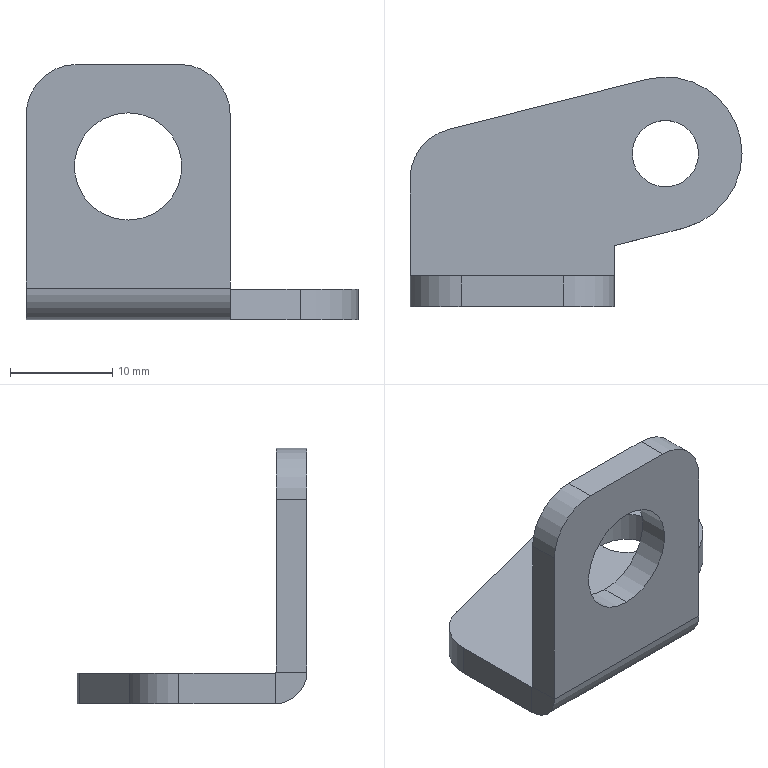Part | SolidWorks | features EdgeFlange 1, Fillet 1, FlatPattern 1, ICE 1, SMBaseFlange 1, SheetMetal 1 | 1 solid | 24 faces | box 32.5 x 22.5 x 25 mm | volume 2512 mm3 | plane 13 | cylinder 11 | commonest cylinder face diameters 10 x3 6.5 x2 10.5 x2 15 x2 0.2 x1 6.2 x1
STEP:
#1=CARTESIAN_POINT('',(0.,0.,6.75));
#2=VERTEX_POINT('',#1);
#3=CARTESIAN_POINT('',(0.,0.,17.25));
#4=VERTEX_POINT('',#3);
#5=CARTESIAN_POINT('',(0.,0.,12.));
#6=DIRECTION('',(0.,1.,0.));
#7=DIRECTION('',(0.,0.,1.));
#8=AXIS2_PLACEMENT_3D('',#5,#6,#7);
#9=CIRCLE('',#8,5.25);
#10=EDGE_CURVE('',#2,#4,#9,.T.);
#11=ORIENTED_EDGE('',*,*,#10,.F.);
#12=CARTESIAN_POINT('',(0.,3.,6.75));
#13=VERTEX_POINT('',#12);
#14=CARTESIAN_POINT('',(0.,-7.,6.75));
#15=DIRECTION('',(0.,1.,0.));
#16=VECTOR('',#15,1000.);
#17=LINE('',#14,#16);
#18=EDGE_CURVE('',#2,#13,#17,.T.);
#19=ORIENTED_EDGE('',*,*,#18,.T.);
#20=CARTESIAN_POINT('',(0.,3.,17.25));
#21=VERTEX_POINT('',#20);
#22=CARTESIAN_POINT('',(0.,3.,12.));
#23=DIRECTION('',(0.,1.,0.));
#24=DIRECTION('',(0.,0.,1.));
#25=AXIS2_PLACEMENT_3D('',#22,#23,#24);
#26=CIRCLE('',#25,5.25);
#27=EDGE_CURVE('',#13,#21,#26,.T.);
#28=ORIENTED_EDGE('',*,*,#27,.T.);
#29=CARTESIAN_POINT('',(0.,-7.,17.25));
#30=DIRECTION('',(0.,1.,0.));
#31=VECTOR('',#30,1000.);
#32=LINE('',#29,#31);
#33=EDGE_CURVE('',#4,#21,#32,.T.);
#34=ORIENTED_EDGE('',*,*,#33,.F.);
#35=EDGE_LOOP('',(#11,#19,#28,#34));
#36=FACE_OUTER_BOUND('',#35,.T.);
#37=CARTESIAN_POINT('',(0.,-7.,12.));
#38=DIRECTION('',(0.,1.,0.));
#39=DIRECTION('',(0.,0.,1.));
#40=AXIS2_PLACEMENT_3D('',#37,#38,#39);
#41=CYLINDRICAL_SURFACE('',#40,5.25);
#42=ADVANCED_FACE('',(#36),#41,.F.);
#43=CARTESIAN_POINT('',(11.75,15.,-3.));
#44=VERTEX_POINT('',#43);
#45=CARTESIAN_POINT('',(18.25,15.,-3.));
#46=VERTEX_POINT('',#45);
#47=CARTESIAN_POINT('',(15.,15.,-3.));
#48=DIRECTION('',(0.,0.,1.));
#49=DIRECTION('',(1.,0.,0.));
#50=AXIS2_PLACEMENT_3D('',#47,#48,#49);
#51=CIRCLE('',#50,3.25);
#52=EDGE_CURVE('',#44,#46,#51,.T.);
#53=ORIENTED_EDGE('',*,*,#52,.F.);
#54=CARTESIAN_POINT('',(11.75,15.,0.));
#55=VERTEX_POINT('',#54);
#56=CARTESIAN_POINT('',(11.75,15.,-3.));
#57=DIRECTION('',(0.,0.,1.));
#58=VECTOR('',#57,1000.);
#59=LINE('',#56,#58);
#60=EDGE_CURVE('',#44,#55,#59,.T.);
#61=ORIENTED_EDGE('',*,*,#60,.T.);
#62=CARTESIAN_POINT('',(18.25,15.,0.));
#63=VERTEX_POINT('',#62);
#64=CARTESIAN_POINT('',(15.,15.,0.));
#65=DIRECTION('',(0.,0.,1.));
#66=DIRECTION('',(1.,0.,0.));
#67=AXIS2_PLACEMENT_3D('',#64,#65,#66);
#68=CIRCLE('',#67,3.25);
#69=EDGE_CURVE('',#55,#63,#68,.T.);
#70=ORIENTED_EDGE('',*,*,#69,.T.);
#71=CARTESIAN_POINT('',(18.25,15.,-3.));
#72=DIRECTION('',(0.,0.,1.));
#73=VECTOR('',#72,1000.);
#74=LINE('',#71,#73);
#75=EDGE_CURVE('',#46,#63,#74,.T.);
#76=ORIENTED_EDGE('',*,*,#75,.F.);
#77=EDGE_LOOP('',(#53,#61,#70,#76));
#78=FACE_OUTER_BOUND('',#77,.T.);
#79=CARTESIAN_POINT('',(15.,15.,-3.));
#80=DIRECTION('',(0.,0.,1.));
#81=DIRECTION('',(1.,0.,0.));
#82=AXIS2_PLACEMENT_3D('',#79,#80,#81);
#83=CYLINDRICAL_SURFACE('',#82,3.25);
#84=ADVANCED_FACE('',(#78),#83,.F.);
#85=CARTESIAN_POINT('',(16.838,7.729,-3.));
#86=VERTEX_POINT('',#85);
#87=CARTESIAN_POINT('',(22.5,15.,-3.));
#88=VERTEX_POINT('',#87);
#89=CARTESIAN_POINT('',(15.,15.,-3.));
#90=DIRECTION('',(0.,0.,1.));
#91=DIRECTION('',(1.,0.,0.));
#92=AXIS2_PLACEMENT_3D('',#89,#90,#91);
#93=CIRCLE('',#92,7.5);
#94=EDGE_CURVE('',#86,#88,#93,.T.);
#95=ORIENTED_EDGE('',*,*,#94,.T.);
#96=CARTESIAN_POINT('',(22.5,15.,0.));
#97=VERTEX_POINT('',#96);
#98=CARTESIAN_POINT('',(22.5,15.,-3.));
#99=DIRECTION('',(0.,0.,1.));
#100=VECTOR('',#99,1000.);
#101=LINE('',#98,#100);
#102=EDGE_CURVE('',#88,#97,#101,.T.);
#103=ORIENTED_EDGE('',*,*,#102,.T.);
#104=CARTESIAN_POINT('',(16.838,7.729,0.));
#105=VERTEX_POINT('',#104);
#106=CARTESIAN_POINT('',(15.,15.,0.));
#107=DIRECTION('',(0.,0.,1.));
#108=DIRECTION('',(1.,0.,0.));
#109=AXIS2_PLACEMENT_3D('',#106,#107,#108);
#110=CIRCLE('',#109,7.5);
#111=EDGE_CURVE('',#105,#97,#110,.T.);
#112=ORIENTED_EDGE('',*,*,#111,.F.);
#113=CARTESIAN_POINT('',(16.838,7.729,-3.));
#114=DIRECTION('',(0.,0.,1.));
#115=VECTOR('',#114,1000.);
#116=LINE('',#113,#115);
#117=EDGE_CURVE('',#86,#105,#116,.T.);
#118=ORIENTED_EDGE('',*,*,#117,.F.);
#119=EDGE_LOOP('',(#95,#103,#112,#118));
#120=FACE_OUTER_BOUND('',#119,.T.);
#121=CARTESIAN_POINT('',(15.,15.,-3.));
#122=DIRECTION('',(0.,0.,1.));
#123=DIRECTION('',(1.,0.,0.));
#124=AXIS2_PLACEMENT_3D('',#121,#122,#123);
#125=CYLINDRICAL_SURFACE('',#124,7.5);
#126=ADVANCED_FACE('',(#120),#125,.T.);
#127=CARTESIAN_POINT('',(10.,3.1,0.));
#128=VERTEX_POINT('',#127);
#129=CARTESIAN_POINT('',(10.,6.,0.));
#130=VERTEX_POINT('',#129);
#131=CARTESIAN_POINT('',(10.,0.,0.));
#132=DIRECTION('',(0.,1.,0.));
#133=VECTOR('',#132,1000.);
#134=LINE('',#131,#133);
#135=EDGE_CURVE('',#128,#130,#134,.T.);
#136=ORIENTED_EDGE('',*,*,#135,.F.);
#137=CARTESIAN_POINT('',(10.,3.1,-3.));
#138=VERTEX_POINT('',#137);
#139=CARTESIAN_POINT('',(10.,3.1,0.));
#140=DIRECTION('',(0.,0.,-1.));
#141=VECTOR('',#140,1000.);
#142=LINE('',#139,#141);
#143=EDGE_CURVE('',#128,#138,#142,.T.);
#144=ORIENTED_EDGE('',*,*,#143,.T.);
#145=CARTESIAN_POINT('',(10.,6.,-3.));
#146=VERTEX_POINT('',#145);
#147=CARTESIAN_POINT('',(10.,0.,-3.));
#148=DIRECTION('',(0.,1.,0.));
#149=VECTOR('',#148,1000.);
#150=LINE('',#147,#149);
#151=EDGE_CURVE('',#138,#146,#150,.T.);
#152=ORIENTED_EDGE('',*,*,#151,.T.);
#153=CARTESIAN_POINT('',(10.,6.,-3.));
#154=DIRECTION('',(0.,0.,1.));
#155=VECTOR('',#154,1000.);
#156=LINE('',#153,#155);
#157=EDGE_CURVE('',#146,#130,#156,.T.);
#158=ORIENTED_EDGE('',*,*,#157,.T.);
#159=EDGE_LOOP('',(#136,#144,#152,#158));
#160=FACE_OUTER_BOUND('',#159,.T.);
#161=CARTESIAN_POINT('',(10.,0.,-3.));
#162=DIRECTION('',(1.,0.,0.));
#163=DIRECTION('',(0.,1.,0.));
#164=AXIS2_PLACEMENT_3D('',#161,#162,#163);
#165=PLANE('',#164);
#166=ADVANCED_FACE('',(#160),#165,.T.);
#167=CARTESIAN_POINT('',(15.,15.,-3.));
#168=DIRECTION('',(0.,0.,1.));
#169=DIRECTION('',(1.,0.,0.));
#170=AXIS2_PLACEMENT_3D('',#167,#168,#169);
#171=CIRCLE('',#170,3.25);
#172=EDGE_CURVE('',#46,#44,#171,.T.);
#173=ORIENTED_EDGE('',*,*,#172,.T.);
#174=ORIENTED_EDGE('',*,*,#52,.T.);
#175=EDGE_LOOP('',(#173,#174));
#176=FACE_BOUND('',#175,.T.);
#177=CARTESIAN_POINT('',(-10.,3.1,-3.));
#178=VERTEX_POINT('',#177);
#179=CARTESIAN_POINT('',(10.,3.1,-3.));
#180=DIRECTION('',(-1.,0.,0.));
#181=VECTOR('',#180,1000.);
#182=LINE('',#179,#181);
#183=EDGE_CURVE('',#138,#178,#182,.T.);
#184=ORIENTED_EDGE('',*,*,#183,.T.);
#185=CARTESIAN_POINT('',(-10.,12.522,-3.));
#186=VERTEX_POINT('',#185);
#187=CARTESIAN_POINT('',(-10.,0.,-3.));
#188=DIRECTION('',(0.,-1.,0.));
#189=VECTOR('',#188,1000.);
#190=LINE('',#187,#189);
#191=EDGE_CURVE('',#186,#178,#190,.T.);
#192=ORIENTED_EDGE('',*,*,#191,.F.);
#193=CARTESIAN_POINT('',(-6.225,17.37,-3.));
#194=VERTEX_POINT('',#193);
#195=CARTESIAN_POINT('',(-5.,12.522,-3.));
#196=DIRECTION('',(0.,0.,1.));
#197=DIRECTION('',(1.,0.,0.));
#198=AXIS2_PLACEMENT_3D('',#195,#196,#197);
#199=CIRCLE('',#198,5.);
#200=EDGE_CURVE('',#194,#186,#199,.T.);
#201=ORIENTED_EDGE('',*,*,#200,.F.);
#202=CARTESIAN_POINT('',(13.162,22.271,-3.));
#203=VERTEX_POINT('',#202);
#204=CARTESIAN_POINT('',(-6.225,17.37,-3.));
#205=DIRECTION('',(-0.9695,-0.2451,0.));
#206=VECTOR('',#205,1000.);
#207=LINE('',#204,#206);
#208=EDGE_CURVE('',#203,#194,#207,.T.);
#209=ORIENTED_EDGE('',*,*,#208,.F.);
#210=CARTESIAN_POINT('',(15.,15.,-3.));
#211=DIRECTION('',(0.,0.,1.));
#212=DIRECTION('',(1.,0.,0.));
#213=AXIS2_PLACEMENT_3D('',#210,#211,#212);
#214=CIRCLE('',#213,7.5);
#215=EDGE_CURVE('',#88,#203,#214,.T.);
#216=ORIENTED_EDGE('',*,*,#215,.F.);
#217=ORIENTED_EDGE('',*,*,#94,.F.);
#218=CARTESIAN_POINT('',(10.,6.,-3.));
#219=DIRECTION('',(0.9695,0.2451,0.));
#220=VECTOR('',#219,1000.);
#221=LINE('',#218,#220);
#222=EDGE_CURVE('',#146,#86,#221,.T.);
#223=ORIENTED_EDGE('',*,*,#222,.F.);
#224=ORIENTED_EDGE('',*,*,#151,.F.);
#225=EDGE_LOOP('',(#184,#192,#201,#209,#216,#217,#223,#224));
#226=FACE_OUTER_BOUND('',#225,.T.);
#227=CARTESIAN_POINT('',(-5.,12.522,-3.));
#228=DIRECTION('',(0.,0.,1.));
#229=DIRECTION('',(1.,0.,0.));
#230=AXIS2_PLACEMENT_3D('',#227,#228,#229);
#231=PLANE('',#230);
#232=ADVANCED_FACE('',(#176,#226),#231,.F.);
#233=CARTESIAN_POINT('',(15.,15.,0.));
#234=DIRECTION('',(0.,0.,1.));
#235=DIRECTION('',(1.,0.,0.));
#236=AXIS2_PLACEMENT_3D('',#233,#234,#235);
#237=CIRCLE('',#236,3.25);
#238=EDGE_CURVE('',#63,#55,#237,.T.);
#239=ORIENTED_EDGE('',*,*,#238,.F.);
#240=ORIENTED_EDGE('',*,*,#69,.F.);
#241=EDGE_LOOP('',(#239,#240));
#242=FACE_BOUND('',#241,.T.);
#243=CARTESIAN_POINT('',(-10.,12.522,0.));
#244=VERTEX_POINT('',#243);
#245=CARTESIAN_POINT('',(-10.,3.1,0.));
#246=VERTEX_POINT('',#245);
#247=CARTESIAN_POINT('',(-10.,0.,0.));
#248=DIRECTION('',(0.,-1.,0.));
#249=VECTOR('',#248,1000.);
#250=LINE('',#247,#249);
#251=EDGE_CURVE('',#244,#246,#250,.T.);
#252=ORIENTED_EDGE('',*,*,#251,.T.);
#253=CARTESIAN_POINT('',(10.,3.1,0.));
#254=DIRECTION('',(-1.,0.,0.));
#255=VECTOR('',#254,1000.);
#256=LINE('',#253,#255);
#257=EDGE_CURVE('',#128,#246,#256,.T.);
#258=ORIENTED_EDGE('',*,*,#257,.F.);
#259=ORIENTED_EDGE('',*,*,#135,.T.);
#260=CARTESIAN_POINT('',(10.,6.,0.));
#261=DIRECTION('',(0.9695,0.2451,0.));
#262=VECTOR('',#261,1000.);
#263=LINE('',#260,#262);
#264=EDGE_CURVE('',#130,#105,#263,.T.);
#265=ORIENTED_EDGE('',*,*,#264,.T.);
#266=ORIENTED_EDGE('',*,*,#111,.T.);
#267=CARTESIAN_POINT('',(13.162,22.271,0.));
#268=VERTEX_POINT('',#267);
#269=CARTESIAN_POINT('',(15.,15.,0.));
#270=DIRECTION('',(0.,0.,1.));
#271=DIRECTION('',(1.,0.,0.));
#272=AXIS2_PLACEMENT_3D('',#269,#270,#271);
#273=CIRCLE('',#272,7.5);
#274=EDGE_CURVE('',#97,#268,#273,.T.);
#275=ORIENTED_EDGE('',*,*,#274,.T.);
#276=CARTESIAN_POINT('',(-6.225,17.37,0.));
#277=VERTEX_POINT('',#276);
#278=CARTESIAN_POINT('',(-6.225,17.37,0.));
#279=DIRECTION('',(-0.9695,-0.2451,0.));
#280=VECTOR('',#279,1000.);
#281=LINE('',#278,#280);
#282=EDGE_CURVE('',#268,#277,#281,.T.);
#283=ORIENTED_EDGE('',*,*,#282,.T.);
#284=CARTESIAN_POINT('',(-5.,12.522,0.));
#285=DIRECTION('',(0.,0.,1.));
#286=DIRECTION('',(1.,0.,0.));
#287=AXIS2_PLACEMENT_3D('',#284,#285,#286);
#288=CIRCLE('',#287,5.);
#289=EDGE_CURVE('',#277,#244,#288,.T.);
#290=ORIENTED_EDGE('',*,*,#289,.T.);
#291=EDGE_LOOP('',(#252,#258,#259,#265,#266,#275,#283,#290));
#292=FACE_OUTER_BOUND('',#291,.T.);
#293=CARTESIAN_POINT('',(-5.,12.522,0.));
#294=DIRECTION('',(0.,0.,1.));
#295=DIRECTION('',(1.,0.,0.));
#296=AXIS2_PLACEMENT_3D('',#293,#294,#295);
#297=PLANE('',#296);
#298=ADVANCED_FACE('',(#242,#292),#297,.T.);
#299=CARTESIAN_POINT('',(-10.,3.1,0.));
#300=DIRECTION('',(0.,0.,-1.));
#301=VECTOR('',#300,1000.);
#302=LINE('',#299,#301);
#303=EDGE_CURVE('',#246,#178,#302,.T.);
#304=ORIENTED_EDGE('',*,*,#303,.F.);
#305=ORIENTED_EDGE('',*,*,#251,.F.);
#306=CARTESIAN_POINT('',(-10.,12.522,-3.));
#307=DIRECTION('',(0.,0.,1.));
#308=VECTOR('',#307,1000.);
#309=LINE('',#306,#308);
#310=EDGE_CURVE('',#186,#244,#309,.T.);
#311=ORIENTED_EDGE('',*,*,#310,.F.);
#312=ORIENTED_EDGE('',*,*,#191,.T.);
#313=EDGE_LOOP('',(#304,#305,#311,#312));
#314=FACE_OUTER_BOUND('',#313,.T.);
#315=CARTESIAN_POINT('',(-10.,0.,-3.));
#316=DIRECTION('',(-1.,0.,0.));
#317=DIRECTION('',(0.,0.,1.));
#318=AXIS2_PLACEMENT_3D('',#315,#316,#317);
#319=PLANE('',#318);
#320=ADVANCED_FACE('',(#314),#319,.T.);
#321=ORIENTED_EDGE('',*,*,#289,.F.);
#322=CARTESIAN_POINT('',(-6.225,17.37,-3.));
#323=DIRECTION('',(0.,0.,1.));
#324=VECTOR('',#323,1000.);
#325=LINE('',#322,#324);
#326=EDGE_CURVE('',#194,#277,#325,.T.);
#327=ORIENTED_EDGE('',*,*,#326,.F.);
#328=ORIENTED_EDGE('',*,*,#200,.T.);
#329=ORIENTED_EDGE('',*,*,#310,.T.);
#330=EDGE_LOOP('',(#321,#327,#328,#329));
#331=FACE_OUTER_BOUND('',#330,.T.);
#332=CARTESIAN_POINT('',(-5.,12.522,-3.));
#333=DIRECTION('',(0.,0.,1.));
#334=DIRECTION('',(1.,0.,0.));
#335=AXIS2_PLACEMENT_3D('',#332,#333,#334);
#336=CYLINDRICAL_SURFACE('',#335,5.);
#337=ADVANCED_FACE('',(#331),#336,.T.);
#338=ORIENTED_EDGE('',*,*,#282,.F.);
#339=CARTESIAN_POINT('',(13.162,22.271,-3.));
#340=DIRECTION('',(0.,0.,1.));
#341=VECTOR('',#340,1000.);
#342=LINE('',#339,#341);
#343=EDGE_CURVE('',#203,#268,#342,.T.);
#344=ORIENTED_EDGE('',*,*,#343,.F.);
#345=ORIENTED_EDGE('',*,*,#208,.T.);
#346=ORIENTED_EDGE('',*,*,#326,.T.);
#347=EDGE_LOOP('',(#338,#344,#345,#346));
#348=FACE_OUTER_BOUND('',#347,.T.);
#349=CARTESIAN_POINT('',(-6.225,17.37,-3.));
#350=DIRECTION('',(-0.2451,0.9695,0.));
#351=DIRECTION('',(-0.9695,-0.2451,0.));
#352=AXIS2_PLACEMENT_3D('',#349,#350,#351);
#353=PLANE('',#352);
#354=ADVANCED_FACE('',(#348),#353,.T.);
#355=ORIENTED_EDGE('',*,*,#102,.F.);
#356=ORIENTED_EDGE('',*,*,#215,.T.);
#357=ORIENTED_EDGE('',*,*,#343,.T.);
#358=ORIENTED_EDGE('',*,*,#274,.F.);
#359=EDGE_LOOP('',(#355,#356,#357,#358));
#360=FACE_OUTER_BOUND('',#359,.T.);
#361=CARTESIAN_POINT('',(15.,15.,-3.));
#362=DIRECTION('',(0.,0.,1.));
#363=DIRECTION('',(1.,0.,0.));
#364=AXIS2_PLACEMENT_3D('',#361,#362,#363);
#365=CYLINDRICAL_SURFACE('',#364,7.5);
#366=ADVANCED_FACE('',(#360),#365,.T.);
#367=ORIENTED_EDGE('',*,*,#264,.F.);
#368=ORIENTED_EDGE('',*,*,#157,.F.);
#369=ORIENTED_EDGE('',*,*,#222,.T.);
#370=ORIENTED_EDGE('',*,*,#117,.T.);
#371=EDGE_LOOP('',(#367,#368,#369,#370));
#372=FACE_OUTER_BOUND('',#371,.T.);
#373=CARTESIAN_POINT('',(10.,6.,-3.));
#374=DIRECTION('',(0.2451,-0.9695,0.));
#375=DIRECTION('',(0.9695,0.2451,0.));
#376=AXIS2_PLACEMENT_3D('',#373,#374,#375);
#377=PLANE('',#376);
#378=ADVANCED_FACE('',(#372),#377,.T.);
#379=ORIENTED_EDGE('',*,*,#60,.F.);
#380=ORIENTED_EDGE('',*,*,#172,.F.);
#381=ORIENTED_EDGE('',*,*,#75,.T.);
#382=ORIENTED_EDGE('',*,*,#238,.T.);
#383=EDGE_LOOP('',(#379,#380,#381,#382));
#384=FACE_OUTER_BOUND('',#383,.T.);
#385=CARTESIAN_POINT('',(15.,15.,-3.));
#386=DIRECTION('',(0.,0.,1.));
#387=DIRECTION('',(1.,0.,0.));
#388=AXIS2_PLACEMENT_3D('',#385,#386,#387);
#389=CYLINDRICAL_SURFACE('',#388,3.25);
#390=ADVANCED_FACE('',(#384),#389,.F.);
#391=CARTESIAN_POINT('',(-10.,3.,0.1));
#392=VERTEX_POINT('',#391);
#393=CARTESIAN_POINT('',(-10.,0.,0.1));
#394=VERTEX_POINT('',#393);
#395=CARTESIAN_POINT('',(-10.,0.,0.1));
#396=DIRECTION('',(0.,-1.,0.));
#397=VECTOR('',#396,1000.);
#398=LINE('',#395,#397);
#399=EDGE_CURVE('',#392,#394,#398,.T.);
#400=ORIENTED_EDGE('',*,*,#399,.F.);
#401=CARTESIAN_POINT('',(-10.,3.1,0.1));
#402=DIRECTION('',(-1.,0.,0.));
#403=DIRECTION('',(0.,0.,-1.));
#404=AXIS2_PLACEMENT_3D('',#401,#402,#403);
#405=CIRCLE('',#404,0.1);
#406=EDGE_CURVE('',#246,#392,#405,.T.);
#407=ORIENTED_EDGE('',*,*,#406,.F.);
#408=ORIENTED_EDGE('',*,*,#303,.T.);
#409=CARTESIAN_POINT('',(-10.,3.1,0.1));
#410=DIRECTION('',(-1.,0.,0.));
#411=DIRECTION('',(0.,0.,-1.));
#412=AXIS2_PLACEMENT_3D('',#409,#410,#411);
#413=CIRCLE('',#412,3.1);
#414=EDGE_CURVE('',#178,#394,#413,.T.);
#415=ORIENTED_EDGE('',*,*,#414,.T.);
#416=EDGE_LOOP('',(#400,#407,#408,#415));
#417=FACE_OUTER_BOUND('',#416,.T.);
#418=CARTESIAN_POINT('',(-10.,3.1,0.1));
#419=DIRECTION('',(-1.,0.,0.));
#420=DIRECTION('',(0.,0.,1.));
#421=AXIS2_PLACEMENT_3D('',#418,#419,#420);
#422=PLANE('',#421);
#423=ADVANCED_FACE('',(#417),#422,.T.);
#424=CARTESIAN_POINT('',(10.,3.,0.1));
#425=VERTEX_POINT('',#424);
#426=CARTESIAN_POINT('',(10.,3.1,0.1));
#427=DIRECTION('',(1.,0.,0.));
#428=DIRECTION('',(0.,0.,-1.));
#429=AXIS2_PLACEMENT_3D('',#426,#427,#428);
#430=CIRCLE('',#429,0.1);
#431=EDGE_CURVE('',#425,#128,#430,.T.);
#432=ORIENTED_EDGE('',*,*,#431,.F.);
#433=CARTESIAN_POINT('',(10.,0.,0.1));
#434=VERTEX_POINT('',#433);
#435=CARTESIAN_POINT('',(10.,3.,0.1));
#436=DIRECTION('',(0.,-1.,0.));
#437=VECTOR('',#436,1000.);
#438=LINE('',#435,#437);
#439=EDGE_CURVE('',#425,#434,#438,.T.);
#440=ORIENTED_EDGE('',*,*,#439,.T.);
#441=CARTESIAN_POINT('',(10.,3.1,0.1));
#442=DIRECTION('',(1.,0.,0.));
#443=DIRECTION('',(0.,0.,-1.));
#444=AXIS2_PLACEMENT_3D('',#441,#442,#443);
#445=CIRCLE('',#444,3.1);
#446=EDGE_CURVE('',#434,#138,#445,.T.);
#447=ORIENTED_EDGE('',*,*,#446,.T.);
#448=ORIENTED_EDGE('',*,*,#143,.F.);
#449=EDGE_LOOP('',(#432,#440,#447,#448));
#450=FACE_OUTER_BOUND('',#449,.T.);
#451=CARTESIAN_POINT('',(10.,3.1,0.1));
#452=DIRECTION('',(-1.,0.,0.));
#453=DIRECTION('',(0.,0.,1.));
#454=AXIS2_PLACEMENT_3D('',#451,#452,#453);
#455=PLANE('',#454);
#456=ADVANCED_FACE('',(#450),#455,.F.);
#457=ORIENTED_EDGE('',*,*,#183,.F.);
#458=ORIENTED_EDGE('',*,*,#446,.F.);
#459=CARTESIAN_POINT('',(-10.,0.,0.1));
#460=DIRECTION('',(-1.,0.,0.));
#461=VECTOR('',#460,1000.);
#462=LINE('',#459,#461);
#463=EDGE_CURVE('',#434,#394,#462,.T.);
#464=ORIENTED_EDGE('',*,*,#463,.T.);
#465=ORIENTED_EDGE('',*,*,#414,.F.);
#466=EDGE_LOOP('',(#457,#458,#464,#465));
#467=FACE_OUTER_BOUND('',#466,.T.);
#468=CARTESIAN_POINT('',(10.,3.1,0.1));
#469=DIRECTION('',(1.,0.,0.));
#470=DIRECTION('',(0.,-1.,0.));
#471=AXIS2_PLACEMENT_3D('',#468,#469,#470);
#472=CYLINDRICAL_SURFACE('',#471,3.1);
#473=ADVANCED_FACE('',(#467),#472,.T.);
#474=ORIENTED_EDGE('',*,*,#257,.T.);
#475=ORIENTED_EDGE('',*,*,#406,.T.);
#476=CARTESIAN_POINT('',(-10.,3.,0.1));
#477=DIRECTION('',(1.,0.,0.));
#478=VECTOR('',#477,1000.);
#479=LINE('',#476,#478);
#480=EDGE_CURVE('',#392,#425,#479,.T.);
#481=ORIENTED_EDGE('',*,*,#480,.T.);
#482=ORIENTED_EDGE('',*,*,#431,.T.);
#483=EDGE_LOOP('',(#474,#475,#481,#482));
#484=FACE_OUTER_BOUND('',#483,.T.);
#485=CARTESIAN_POINT('',(10.,3.1,0.1));
#486=DIRECTION('',(1.,0.,0.));
#487=DIRECTION('',(0.,-1.,0.));
#488=AXIS2_PLACEMENT_3D('',#485,#486,#487);
#489=CYLINDRICAL_SURFACE('',#488,0.1);
#490=ADVANCED_FACE('',(#484),#489,.F.);
#491=CARTESIAN_POINT('',(-10.,0.,17.));
#492=VERTEX_POINT('',#491);
#493=CARTESIAN_POINT('',(-10.,0.,0.));
#494=DIRECTION('',(0.,0.,-1.));
#495=VECTOR('',#494,1000.);
#496=LINE('',#493,#495);
#497=EDGE_CURVE('',#492,#394,#496,.T.);
#498=ORIENTED_EDGE('',*,*,#497,.F.);
#499=CARTESIAN_POINT('',(-10.,3.,17.));
#500=VERTEX_POINT('',#499);
#501=CARTESIAN_POINT('',(-10.,0.,17.));
#502=DIRECTION('',(0.,1.,0.));
#503=VECTOR('',#502,1000.);
#504=LINE('',#501,#503);
#505=EDGE_CURVE('',#492,#500,#504,.T.);
#506=ORIENTED_EDGE('',*,*,#505,.T.);
#507=CARTESIAN_POINT('',(-10.,3.,0.));
#508=DIRECTION('',(0.,0.,-1.));
#509=VECTOR('',#508,1000.);
#510=LINE('',#507,#509);
#511=EDGE_CURVE('',#500,#392,#510,.T.);
#512=ORIENTED_EDGE('',*,*,#511,.T.);
#513=ORIENTED_EDGE('',*,*,#399,.T.);
#514=EDGE_LOOP('',(#498,#506,#512,#513));
#515=FACE_OUTER_BOUND('',#514,.T.);
#516=CARTESIAN_POINT('',(-10.,0.,0.));
#517=DIRECTION('',(1.,0.,0.));
#518=DIRECTION('',(0.,0.,-1.));
#519=AXIS2_PLACEMENT_3D('',#516,#517,#518);
#520=PLANE('',#519);
#521=ADVANCED_FACE('',(#515),#520,.F.);
#522=CARTESIAN_POINT('',(10.,3.,17.));
#523=VERTEX_POINT('',#522);
#524=CARTESIAN_POINT('',(10.,3.,22.));
#525=DIRECTION('',(0.,0.,1.));
#526=VECTOR('',#525,1000.);
#527=LINE('',#524,#526);
#528=EDGE_CURVE('',#425,#523,#527,.T.);
#529=ORIENTED_EDGE('',*,*,#528,.T.);
#530=CARTESIAN_POINT('',(10.,0.,17.));
#531=VERTEX_POINT('',#530);
#532=CARTESIAN_POINT('',(10.,0.,17.));
#533=DIRECTION('',(0.,-1.,0.));
#534=VECTOR('',#533,1000.);
#535=LINE('',#532,#534);
#536=EDGE_CURVE('',#523,#531,#535,.T.);
#537=ORIENTED_EDGE('',*,*,#536,.T.);
#538=CARTESIAN_POINT('',(10.,0.,0.));
#539=DIRECTION('',(0.,0.,1.));
#540=VECTOR('',#539,1000.);
#541=LINE('',#538,#540);
#542=EDGE_CURVE('',#434,#531,#541,.T.);
#543=ORIENTED_EDGE('',*,*,#542,.F.);
#544=ORIENTED_EDGE('',*,*,#439,.F.);
#545=EDGE_LOOP('',(#529,#537,#543,#544));
#546=FACE_OUTER_BOUND('',#545,.T.);
#547=CARTESIAN_POINT('',(10.,0.,22.));
#548=DIRECTION('',(-1.,0.,0.));
#549=DIRECTION('',(0.,0.,1.));
#550=AXIS2_PLACEMENT_3D('',#547,#548,#549);
#551=PLANE('',#550);
#552=ADVANCED_FACE('',(#546),#551,.F.);
#553=CARTESIAN_POINT('',(0.,0.,12.));
#554=DIRECTION('',(0.,1.,0.));
#555=DIRECTION('',(0.,0.,1.));
#556=AXIS2_PLACEMENT_3D('',#553,#554,#555);
#557=CIRCLE('',#556,5.25);
#558=EDGE_CURVE('',#4,#2,#557,.T.);
#559=ORIENTED_EDGE('',*,*,#558,.T.);
#560=ORIENTED_EDGE('',*,*,#10,.T.);
#561=EDGE_LOOP('',(#559,#560));
#562=FACE_BOUND('',#561,.T.);
#563=ORIENTED_EDGE('',*,*,#542,.T.);
#564=CARTESIAN_POINT('',(5.,0.,22.));
#565=VERTEX_POINT('',#564);
#566=CARTESIAN_POINT('',(5.,0.,17.));
#567=DIRECTION('',(0.,-1.,0.));
#568=DIRECTION('',(0.,0.,1.));
#569=AXIS2_PLACEMENT_3D('',#566,#567,#568);
#570=CIRCLE('',#569,5.);
#571=EDGE_CURVE('',#531,#565,#570,.T.);
#572=ORIENTED_EDGE('',*,*,#571,.T.);
#573=CARTESIAN_POINT('',(-5.,0.,22.));
#574=VERTEX_POINT('',#573);
#575=CARTESIAN_POINT('',(0.,0.,22.));
#576=DIRECTION('',(-1.,0.,0.));
#577=VECTOR('',#576,1000.);
#578=LINE('',#575,#577);
#579=EDGE_CURVE('',#565,#574,#578,.T.);
#580=ORIENTED_EDGE('',*,*,#579,.T.);
#581=CARTESIAN_POINT('',(-5.,0.,17.));
#582=DIRECTION('',(0.,-1.,0.));
#583=DIRECTION('',(0.,0.,1.));
#584=AXIS2_PLACEMENT_3D('',#581,#582,#583);
#585=CIRCLE('',#584,5.);
#586=EDGE_CURVE('',#574,#492,#585,.T.);
#587=ORIENTED_EDGE('',*,*,#586,.T.);
#588=ORIENTED_EDGE('',*,*,#497,.T.);
#589=ORIENTED_EDGE('',*,*,#463,.F.);
#590=EDGE_LOOP('',(#563,#572,#580,#587,#588,#589));
#591=FACE_OUTER_BOUND('',#590,.T.);
#592=CARTESIAN_POINT('',(0.,0.,0.));
#593=DIRECTION('',(0.,1.,0.));
#594=DIRECTION('',(0.,0.,1.));
#595=AXIS2_PLACEMENT_3D('',#592,#593,#594);
#596=PLANE('',#595);
#597=ADVANCED_FACE('',(#562,#591),#596,.F.);
#598=CARTESIAN_POINT('',(0.,3.,12.));
#599=DIRECTION('',(0.,1.,0.));
#600=DIRECTION('',(0.,0.,1.));
#601=AXIS2_PLACEMENT_3D('',#598,#599,#600);
#602=CIRCLE('',#601,5.25);
#603=EDGE_CURVE('',#21,#13,#602,.T.);
#604=ORIENTED_EDGE('',*,*,#603,.F.);
#605=ORIENTED_EDGE('',*,*,#27,.F.);
#606=EDGE_LOOP('',(#604,#605));
#607=FACE_BOUND('',#606,.T.);
#608=CARTESIAN_POINT('',(5.,3.,22.));
#609=VERTEX_POINT('',#608);
#610=CARTESIAN_POINT('',(-5.,3.,22.));
#611=VERTEX_POINT('',#610);
#612=CARTESIAN_POINT('',(-10.,3.,22.));
#613=DIRECTION('',(-1.,0.,0.));
#614=VECTOR('',#613,1000.);
#615=LINE('',#612,#614);
#616=EDGE_CURVE('',#609,#611,#615,.T.);
#617=ORIENTED_EDGE('',*,*,#616,.F.);
#618=CARTESIAN_POINT('',(5.,3.,17.));
#619=DIRECTION('',(0.,1.,0.));
#620=DIRECTION('',(0.,0.,1.));
#621=AXIS2_PLACEMENT_3D('',#618,#619,#620);
#622=CIRCLE('',#621,5.);
#623=EDGE_CURVE('',#609,#523,#622,.T.);
#624=ORIENTED_EDGE('',*,*,#623,.T.);
#625=ORIENTED_EDGE('',*,*,#528,.F.);
#626=ORIENTED_EDGE('',*,*,#480,.F.);
#627=ORIENTED_EDGE('',*,*,#511,.F.);
#628=CARTESIAN_POINT('',(-5.,3.,17.));
#629=DIRECTION('',(0.,1.,0.));
#630=DIRECTION('',(0.,0.,1.));
#631=AXIS2_PLACEMENT_3D('',#628,#629,#630);
#632=CIRCLE('',#631,5.);
#633=EDGE_CURVE('',#500,#611,#632,.T.);
#634=ORIENTED_EDGE('',*,*,#633,.T.);
#635=EDGE_LOOP('',(#617,#624,#625,#626,#627,#634));
#636=FACE_OUTER_BOUND('',#635,.T.);
#637=CARTESIAN_POINT('',(0.,3.,0.));
#638=DIRECTION('',(0.,1.,0.));
#639=DIRECTION('',(0.,0.,1.));
#640=AXIS2_PLACEMENT_3D('',#637,#638,#639);
#641=PLANE('',#640);
#642=ADVANCED_FACE('',(#607,#636),#641,.T.);
#643=ORIENTED_EDGE('',*,*,#579,.F.);
#644=CARTESIAN_POINT('',(5.,0.,22.));
#645=DIRECTION('',(0.,1.,0.));
#646=VECTOR('',#645,1000.);
#647=LINE('',#644,#646);
#648=EDGE_CURVE('',#565,#609,#647,.T.);
#649=ORIENTED_EDGE('',*,*,#648,.T.);
#650=ORIENTED_EDGE('',*,*,#616,.T.);
#651=CARTESIAN_POINT('',(-5.,0.,22.));
#652=DIRECTION('',(0.,-1.,0.));
#653=VECTOR('',#652,1000.);
#654=LINE('',#651,#653);
#655=EDGE_CURVE('',#611,#574,#654,.T.);
#656=ORIENTED_EDGE('',*,*,#655,.T.);
#657=EDGE_LOOP('',(#643,#649,#650,#656));
#658=FACE_OUTER_BOUND('',#657,.T.);
#659=CARTESIAN_POINT('',(-10.,0.,22.));
#660=DIRECTION('',(0.,0.,-1.));
#661=DIRECTION('',(0.,1.,0.));
#662=AXIS2_PLACEMENT_3D('',#659,#660,#661);
#663=PLANE('',#662);
#664=ADVANCED_FACE('',(#658),#663,.F.);
#665=ORIENTED_EDGE('',*,*,#571,.F.);
#666=ORIENTED_EDGE('',*,*,#536,.F.);
#667=ORIENTED_EDGE('',*,*,#623,.F.);
#668=ORIENTED_EDGE('',*,*,#648,.F.);
#669=EDGE_LOOP('',(#665,#666,#667,#668));
#670=FACE_OUTER_BOUND('',#669,.T.);
#671=CARTESIAN_POINT('',(5.,0.,17.));
#672=DIRECTION('',(0.,1.,0.));
#673=DIRECTION('',(0.,0.,1.));
#674=AXIS2_PLACEMENT_3D('',#671,#672,#673);
#675=CYLINDRICAL_SURFACE('',#674,5.);
#676=ADVANCED_FACE('',(#670),#675,.T.);
#677=ORIENTED_EDGE('',*,*,#586,.F.);
#678=ORIENTED_EDGE('',*,*,#655,.F.);
#679=ORIENTED_EDGE('',*,*,#633,.F.);
#680=ORIENTED_EDGE('',*,*,#505,.F.);
#681=EDGE_LOOP('',(#677,#678,#679,#680));
#682=FACE_OUTER_BOUND('',#681,.T.);
#683=CARTESIAN_POINT('',(-5.,0.,17.));
#684=DIRECTION('',(0.,1.,0.));
#685=DIRECTION('',(0.,0.,1.));
#686=AXIS2_PLACEMENT_3D('',#683,#684,#685);
#687=CYLINDRICAL_SURFACE('',#686,5.);
#688=ADVANCED_FACE('',(#682),#687,.T.);
#689=ORIENTED_EDGE('',*,*,#18,.F.);
#690=ORIENTED_EDGE('',*,*,#558,.F.);
#691=ORIENTED_EDGE('',*,*,#33,.T.);
#692=ORIENTED_EDGE('',*,*,#603,.T.);
#693=EDGE_LOOP('',(#689,#690,#691,#692));
#694=FACE_OUTER_BOUND('',#693,.T.);
#695=CARTESIAN_POINT('',(0.,-7.,12.));
#696=DIRECTION('',(0.,1.,0.));
#697=DIRECTION('',(0.,0.,1.));
#698=AXIS2_PLACEMENT_3D('',#695,#696,#697);
#699=CYLINDRICAL_SURFACE('',#698,5.25);
#700=ADVANCED_FACE('',(#694),#699,.F.);
#701=CLOSED_SHELL('',(#42,#84,#126,#166,#232,#298,#320,#337,#354,#366,#378,#390,#423,#456,#473,#490,#521,#552,#597,#642,#664,#676,#688,#700));
#702=MANIFOLD_SOLID_BREP('',#701);
#703=CARTESIAN_POINT('',(0.,0.,0.));
#704=DIRECTION('',(0.,0.,1.));
#705=DIRECTION('',(1.,0.,0.));
#706=AXIS2_PLACEMENT_3D('',#703,#704,#705);
#707=(LENGTH_UNIT()NAMED_UNIT(*)SI_UNIT(.MILLI.,.METRE.));
#708=UNCERTAINTY_MEASURE_WITH_UNIT(LENGTH_MEASURE(0.00001),#707,'','');
#709=(NAMED_UNIT(*)PLANE_ANGLE_UNIT()SI_UNIT($,.RADIAN.));
#710=(NAMED_UNIT(*)SI_UNIT($,.STERADIAN.)SOLID_ANGLE_UNIT());
#711=(GEOMETRIC_REPRESENTATION_CONTEXT(3)GLOBAL_UNCERTAINTY_ASSIGNED_CONTEXT((#708))GLOBAL_UNIT_ASSIGNED_CONTEXT((#707,#709,#710))REPRESENTATION_CONTEXT('',''));
#712=ADVANCED_BREP_SHAPE_REPRESENTATION('',(#702,#706),#711);